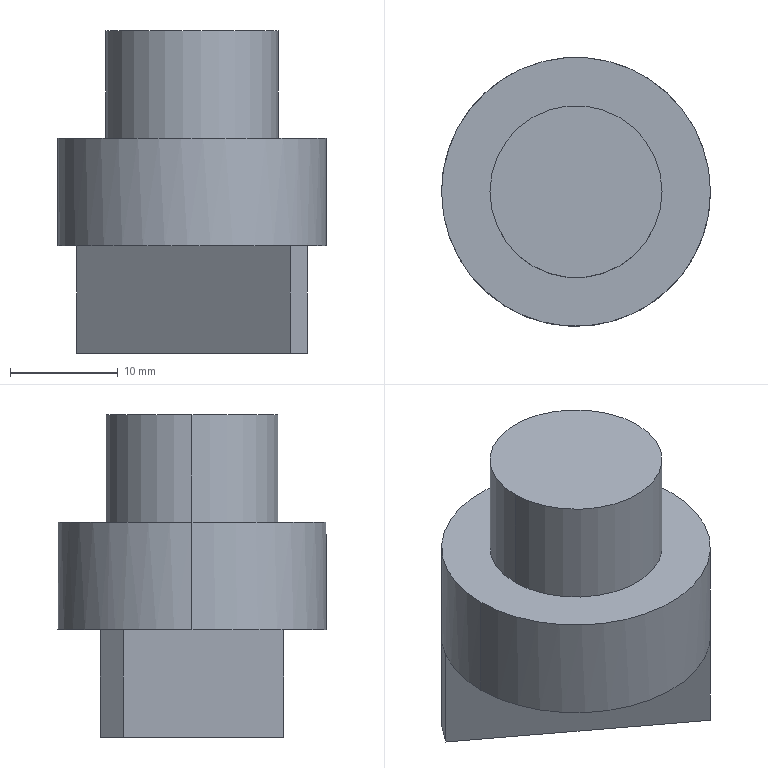Part | STEP file | Selector switch | 1 solid | 15 faces | box 25 x 25 x 30 mm | volume 7576 mm3 | plane 11 | cylinder 4 | commonest cylinder face diameters 16 x2 25 x2
STEP:
#1=CARTESIAN_POINT('',(0.,0.,0.));
#2=DIRECTION('',(0.,0.,1.));
#3=DIRECTION('',(1.,0.,0.));
#4=AXIS2_PLACEMENT_3D('',#1,#2,#3);
#5=CARTESIAN_POINT('',(-12.5,0.,10.));
#6=VERTEX_POINT('',#5);
#7=CARTESIAN_POINT('',(12.5,0.,10.));
#8=VERTEX_POINT('',#7);
#9=CARTESIAN_POINT('',(0.,0.,10.));
#10=DIRECTION('',(0.,0.,-1.));
#11=DIRECTION('',(-1.,0.,0.));
#12=AXIS2_PLACEMENT_3D('',#9,#10,#11);
#13=CIRCLE('',#12,12.5);
#14=CARTESIAN_POINT('',(0.,0.,10.));
#15=DIRECTION('',(0.,0.,-1.));
#16=DIRECTION('',(-1.,0.,0.));
#17=AXIS2_PLACEMENT_3D('',#14,#15,#16);
#18=CYLINDRICAL_SURFACE('',#17,12.5);
#19=CARTESIAN_POINT('',(0.,0.));
#20=DIRECTION('',(1.,0.));
#21=VECTOR('',#20,1.);
#22=LINE('',#19,#21);
#23=(GEOMETRIC_REPRESENTATION_CONTEXT(2)PARAMETRIC_REPRESENTATION_CONTEXT()REPRESENTATION_CONTEXT('',''));
#24=DEFINITIONAL_REPRESENTATION('',(#22),#23);
#25=PCURVE('',#18,#24);
#26=CARTESIAN_POINT('',(0.,0.,10.));
#27=DIRECTION('',(0.,0.,1.));
#28=DIRECTION('',(1.,0.,0.));
#29=AXIS2_PLACEMENT_3D('',#26,#27,#28);
#30=PLANE('',#29);
#31=CARTESIAN_POINT('',(-12.5,0.));
#32=CARTESIAN_POINT('',(-12.5,21.651));
#33=CARTESIAN_POINT('',(6.25,10.825));
#34=CARTESIAN_POINT('',(25.,0.));
#35=CARTESIAN_POINT('',(6.25,-10.825));
#36=CARTESIAN_POINT('',(-12.5,-21.651));
#37=CARTESIAN_POINT('',(-12.5,0.));
#38=(BOUNDED_CURVE()B_SPLINE_CURVE(2,(#31,#32,#33,#34,#35,#36,#37),.UNSPECIFIED.,.T.,.F.)B_SPLINE_CURVE_WITH_KNOTS((1,2,2,2,2,1),(-2.094,0.,2.094,4.189,6.283,8.378),.UNSPECIFIED.)CURVE()GEOMETRIC_REPRESENTATION_ITEM()RATIONAL_B_SPLINE_CURVE((1.,0.5,1.,0.5,1.,0.5,1.))REPRESENTATION_ITEM(''));
#39=(GEOMETRIC_REPRESENTATION_CONTEXT(2)PARAMETRIC_REPRESENTATION_CONTEXT()REPRESENTATION_CONTEXT('',''));
#40=DEFINITIONAL_REPRESENTATION('',(#38),#39);
#41=PCURVE('',#30,#40);
#42=SURFACE_CURVE('',#13,(#25,#41),.PCURVE_S1.);
#43=EDGE_CURVE('',#6,#8,#42,.T.);
#44=ORIENTED_EDGE('',*,*,#43,.T.);
#45=CARTESIAN_POINT('',(12.5,0.,0.));
#46=VERTEX_POINT('',#45);
#47=CARTESIAN_POINT('',(12.5,0.,10.));
#48=DIRECTION('',(0.,0.,-1.));
#49=VECTOR('',#48,1.);
#50=LINE('',#47,#49);
#51=CARTESIAN_POINT('',(3.142,0.));
#52=DIRECTION('',(0.,1.));
#53=VECTOR('',#52,1.);
#54=LINE('',#51,#53);
#55=(GEOMETRIC_REPRESENTATION_CONTEXT(2)PARAMETRIC_REPRESENTATION_CONTEXT()REPRESENTATION_CONTEXT('',''));
#56=DEFINITIONAL_REPRESENTATION('',(#54),#55);
#57=PCURVE('',#18,#56);
#58=CARTESIAN_POINT('',(0.,0.,10.));
#59=DIRECTION('',(0.,0.,-1.));
#60=DIRECTION('',(-1.,0.,0.));
#61=AXIS2_PLACEMENT_3D('',#58,#59,#60);
#62=CYLINDRICAL_SURFACE('',#61,12.5);
#63=CARTESIAN_POINT('',(3.142,0.));
#64=DIRECTION('',(0.,1.));
#65=VECTOR('',#64,1.);
#66=LINE('',#63,#65);
#67=(GEOMETRIC_REPRESENTATION_CONTEXT(2)PARAMETRIC_REPRESENTATION_CONTEXT()REPRESENTATION_CONTEXT('',''));
#68=DEFINITIONAL_REPRESENTATION('',(#66),#67);
#69=PCURVE('',#62,#68);
#70=SURFACE_CURVE('',#50,(#57,#69),.PCURVE_S1.);
#71=EDGE_CURVE('',#8,#46,#70,.T.);
#72=ORIENTED_EDGE('',*,*,#71,.T.);
#73=CARTESIAN_POINT('',(-9.149,8.518,0.));
#74=VERTEX_POINT('',#73);
#75=CARTESIAN_POINT('',(0.,0.,0.));
#76=DIRECTION('',(0.,0.,1.));
#77=DIRECTION('',(-1.,0.,0.));
#78=AXIS2_PLACEMENT_3D('',#75,#76,#77);
#79=CIRCLE('',#78,12.5);
#80=CARTESIAN_POINT('',(6.283,10.));
#81=DIRECTION('',(-1.,0.));
#82=VECTOR('',#81,1.);
#83=LINE('',#80,#82);
#84=(GEOMETRIC_REPRESENTATION_CONTEXT(2)PARAMETRIC_REPRESENTATION_CONTEXT()REPRESENTATION_CONTEXT('',''));
#85=DEFINITIONAL_REPRESENTATION('',(#83),#84);
#86=PCURVE('',#18,#85);
#87=CARTESIAN_POINT('',(0.,0.,0.));
#88=DIRECTION('',(0.,0.,1.));
#89=DIRECTION('',(1.,0.,0.));
#90=AXIS2_PLACEMENT_3D('',#87,#88,#89);
#91=PLANE('',#90);
#92=CARTESIAN_POINT('',(0.,0.));
#93=DIRECTION('',(-1.,0.));
#94=AXIS2_PLACEMENT_2D('',#92,#93);
#95=CIRCLE('',#94,12.5);
#96=(GEOMETRIC_REPRESENTATION_CONTEXT(2)PARAMETRIC_REPRESENTATION_CONTEXT()REPRESENTATION_CONTEXT('',''));
#97=DEFINITIONAL_REPRESENTATION('',(#95),#96);
#98=PCURVE('',#91,#97);
#99=SURFACE_CURVE('',#79,(#86,#98),.PCURVE_S1.);
#100=EDGE_CURVE('',#46,#74,#99,.T.);
#101=ORIENTED_EDGE('',*,*,#100,.T.);
#102=CARTESIAN_POINT('',(-10.733,6.406,0.));
#103=VERTEX_POINT('',#102);
#104=CARTESIAN_POINT('',(0.,0.,0.));
#105=DIRECTION('',(0.,0.,1.));
#106=DIRECTION('',(-1.,0.,0.));
#107=AXIS2_PLACEMENT_3D('',#104,#105,#106);
#108=CIRCLE('',#107,12.5);
#109=CARTESIAN_POINT('',(6.283,10.));
#110=DIRECTION('',(-1.,0.));
#111=VECTOR('',#110,1.);
#112=LINE('',#109,#111);
#113=(GEOMETRIC_REPRESENTATION_CONTEXT(2)PARAMETRIC_REPRESENTATION_CONTEXT()REPRESENTATION_CONTEXT('',''));
#114=DEFINITIONAL_REPRESENTATION('',(#112),#113);
#115=PCURVE('',#18,#114);
#116=CARTESIAN_POINT('',(0.,0.,0.));
#117=DIRECTION('',(0.,0.,1.));
#118=DIRECTION('',(1.,0.,0.));
#119=AXIS2_PLACEMENT_3D('',#116,#117,#118);
#120=PLANE('',#119);
#121=CARTESIAN_POINT('',(0.,0.));
#122=DIRECTION('',(-1.,0.));
#123=AXIS2_PLACEMENT_2D('',#121,#122);
#124=CIRCLE('',#123,12.5);
#125=(GEOMETRIC_REPRESENTATION_CONTEXT(2)PARAMETRIC_REPRESENTATION_CONTEXT()REPRESENTATION_CONTEXT('',''));
#126=DEFINITIONAL_REPRESENTATION('',(#124),#125);
#127=PCURVE('',#120,#126);
#128=SURFACE_CURVE('',#108,(#115,#127),.PCURVE_S1.);
#129=EDGE_CURVE('',#74,#103,#128,.T.);
#130=ORIENTED_EDGE('',*,*,#129,.T.);
#131=CARTESIAN_POINT('',(-12.5,0.,0.));
#132=VERTEX_POINT('',#131);
#133=CARTESIAN_POINT('',(0.,0.,0.));
#134=DIRECTION('',(0.,0.,1.));
#135=DIRECTION('',(-1.,0.,0.));
#136=AXIS2_PLACEMENT_3D('',#133,#134,#135);
#137=CIRCLE('',#136,12.5);
#138=CARTESIAN_POINT('',(6.283,10.));
#139=DIRECTION('',(-1.,0.));
#140=VECTOR('',#139,1.);
#141=LINE('',#138,#140);
#142=(GEOMETRIC_REPRESENTATION_CONTEXT(2)PARAMETRIC_REPRESENTATION_CONTEXT()REPRESENTATION_CONTEXT('',''));
#143=DEFINITIONAL_REPRESENTATION('',(#141),#142);
#144=PCURVE('',#18,#143);
#145=CARTESIAN_POINT('',(0.,0.,0.));
#146=DIRECTION('',(0.,0.,1.));
#147=DIRECTION('',(1.,0.,0.));
#148=AXIS2_PLACEMENT_3D('',#145,#146,#147);
#149=PLANE('',#148);
#150=CARTESIAN_POINT('',(0.,0.));
#151=DIRECTION('',(-1.,0.));
#152=AXIS2_PLACEMENT_2D('',#150,#151);
#153=CIRCLE('',#152,12.5);
#154=(GEOMETRIC_REPRESENTATION_CONTEXT(2)PARAMETRIC_REPRESENTATION_CONTEXT()REPRESENTATION_CONTEXT('',''));
#155=DEFINITIONAL_REPRESENTATION('',(#153),#154);
#156=PCURVE('',#149,#155);
#157=SURFACE_CURVE('',#137,(#144,#156),.PCURVE_S1.);
#158=EDGE_CURVE('',#103,#132,#157,.T.);
#159=ORIENTED_EDGE('',*,*,#158,.T.);
#160=CARTESIAN_POINT('',(-12.5,0.,10.));
#161=DIRECTION('',(0.,0.,-1.));
#162=VECTOR('',#161,1.);
#163=LINE('',#160,#162);
#164=CARTESIAN_POINT('',(0.,0.));
#165=DIRECTION('',(0.,1.));
#166=VECTOR('',#165,1.);
#167=LINE('',#164,#166);
#168=(GEOMETRIC_REPRESENTATION_CONTEXT(2)PARAMETRIC_REPRESENTATION_CONTEXT()REPRESENTATION_CONTEXT('',''));
#169=DEFINITIONAL_REPRESENTATION('',(#167),#168);
#170=PCURVE('',#18,#169);
#171=CARTESIAN_POINT('',(6.283,0.));
#172=DIRECTION('',(0.,1.));
#173=VECTOR('',#172,1.);
#174=LINE('',#171,#173);
#175=(GEOMETRIC_REPRESENTATION_CONTEXT(2)PARAMETRIC_REPRESENTATION_CONTEXT()REPRESENTATION_CONTEXT('',''));
#176=DEFINITIONAL_REPRESENTATION('',(#174),#175);
#177=PCURVE('',#62,#176);
#178=SURFACE_CURVE('',#163,(#170,#177),.PCURVE_S1.);
#179=EDGE_CURVE('',#6,#132,#178,.T.);
#180=ORIENTED_EDGE('',*,*,#179,.F.);
#181=EDGE_LOOP('',(#44,#72,#101,#130,#159,#180));
#182=FACE_BOUND('',#181,.T.);
#183=ADVANCED_FACE('',(#182),#18,.T.);
#184=CARTESIAN_POINT('',(-8.,0.,20.));
#185=VERTEX_POINT('',#184);
#186=CARTESIAN_POINT('',(8.,0.,20.));
#187=VERTEX_POINT('',#186);
#188=CARTESIAN_POINT('',(0.,0.,20.));
#189=DIRECTION('',(0.,0.,-1.));
#190=DIRECTION('',(-1.,0.,0.));
#191=AXIS2_PLACEMENT_3D('',#188,#189,#190);
#192=CIRCLE('',#191,8.);
#193=CARTESIAN_POINT('',(0.,0.,20.));
#194=DIRECTION('',(0.,0.,-1.));
#195=DIRECTION('',(-1.,0.,0.));
#196=AXIS2_PLACEMENT_3D('',#193,#194,#195);
#197=CYLINDRICAL_SURFACE('',#196,8.);
#198=CARTESIAN_POINT('',(0.,0.));
#199=DIRECTION('',(1.,0.));
#200=VECTOR('',#199,1.);
#201=LINE('',#198,#200);
#202=(GEOMETRIC_REPRESENTATION_CONTEXT(2)PARAMETRIC_REPRESENTATION_CONTEXT()REPRESENTATION_CONTEXT('',''));
#203=DEFINITIONAL_REPRESENTATION('',(#201),#202);
#204=PCURVE('',#197,#203);
#205=CARTESIAN_POINT('',(0.,0.,20.));
#206=DIRECTION('',(0.,0.,1.));
#207=DIRECTION('',(1.,0.,0.));
#208=AXIS2_PLACEMENT_3D('',#205,#206,#207);
#209=PLANE('',#208);
#210=CARTESIAN_POINT('',(-8.,0.));
#211=CARTESIAN_POINT('',(-8.,13.856));
#212=CARTESIAN_POINT('',(4.,6.928));
#213=CARTESIAN_POINT('',(16.,0.));
#214=CARTESIAN_POINT('',(4.,-6.928));
#215=CARTESIAN_POINT('',(-8.,-13.856));
#216=CARTESIAN_POINT('',(-8.,0.));
#217=(BOUNDED_CURVE()B_SPLINE_CURVE(2,(#210,#211,#212,#213,#214,#215,#216),.UNSPECIFIED.,.T.,.F.)B_SPLINE_CURVE_WITH_KNOTS((1,2,2,2,2,1),(-2.094,0.,2.094,4.189,6.283,8.378),.UNSPECIFIED.)CURVE()GEOMETRIC_REPRESENTATION_ITEM()RATIONAL_B_SPLINE_CURVE((1.,0.5,1.,0.5,1.,0.5,1.))REPRESENTATION_ITEM(''));
#218=(GEOMETRIC_REPRESENTATION_CONTEXT(2)PARAMETRIC_REPRESENTATION_CONTEXT()REPRESENTATION_CONTEXT('',''));
#219=DEFINITIONAL_REPRESENTATION('',(#217),#218);
#220=PCURVE('',#209,#219);
#221=SURFACE_CURVE('',#192,(#204,#220),.PCURVE_S1.);
#222=EDGE_CURVE('',#185,#187,#221,.T.);
#223=ORIENTED_EDGE('',*,*,#222,.T.);
#224=CARTESIAN_POINT('',(8.,0.,10.));
#225=VERTEX_POINT('',#224);
#226=CARTESIAN_POINT('',(8.,0.,20.));
#227=DIRECTION('',(0.,0.,-1.));
#228=VECTOR('',#227,1.);
#229=LINE('',#226,#228);
#230=CARTESIAN_POINT('',(3.142,0.));
#231=DIRECTION('',(0.,1.));
#232=VECTOR('',#231,1.);
#233=LINE('',#230,#232);
#234=(GEOMETRIC_REPRESENTATION_CONTEXT(2)PARAMETRIC_REPRESENTATION_CONTEXT()REPRESENTATION_CONTEXT('',''));
#235=DEFINITIONAL_REPRESENTATION('',(#233),#234);
#236=PCURVE('',#197,#235);
#237=CARTESIAN_POINT('',(0.,0.,20.));
#238=DIRECTION('',(0.,0.,-1.));
#239=DIRECTION('',(-1.,0.,0.));
#240=AXIS2_PLACEMENT_3D('',#237,#238,#239);
#241=CYLINDRICAL_SURFACE('',#240,8.);
#242=CARTESIAN_POINT('',(3.142,0.));
#243=DIRECTION('',(0.,1.));
#244=VECTOR('',#243,1.);
#245=LINE('',#242,#244);
#246=(GEOMETRIC_REPRESENTATION_CONTEXT(2)PARAMETRIC_REPRESENTATION_CONTEXT()REPRESENTATION_CONTEXT('',''));
#247=DEFINITIONAL_REPRESENTATION('',(#245),#246);
#248=PCURVE('',#241,#247);
#249=SURFACE_CURVE('',#229,(#236,#248),.PCURVE_S1.);
#250=EDGE_CURVE('',#187,#225,#249,.T.);
#251=ORIENTED_EDGE('',*,*,#250,.T.);
#252=CARTESIAN_POINT('',(-8.,0.,10.));
#253=VERTEX_POINT('',#252);
#254=CARTESIAN_POINT('',(0.,0.,10.));
#255=DIRECTION('',(0.,0.,-1.));
#256=DIRECTION('',(-1.,0.,0.));
#257=AXIS2_PLACEMENT_3D('',#254,#255,#256);
#258=CIRCLE('',#257,8.);
#259=CARTESIAN_POINT('',(0.,10.));
#260=DIRECTION('',(1.,0.));
#261=VECTOR('',#260,1.);
#262=LINE('',#259,#261);
#263=(GEOMETRIC_REPRESENTATION_CONTEXT(2)PARAMETRIC_REPRESENTATION_CONTEXT()REPRESENTATION_CONTEXT('',''));
#264=DEFINITIONAL_REPRESENTATION('',(#262),#263);
#265=PCURVE('',#197,#264);
#266=CARTESIAN_POINT('',(-8.,0.));
#267=CARTESIAN_POINT('',(-8.,13.856));
#268=CARTESIAN_POINT('',(4.,6.928));
#269=CARTESIAN_POINT('',(16.,0.));
#270=CARTESIAN_POINT('',(4.,-6.928));
#271=CARTESIAN_POINT('',(-8.,-13.856));
#272=CARTESIAN_POINT('',(-8.,0.));
#273=(BOUNDED_CURVE()B_SPLINE_CURVE(2,(#266,#267,#268,#269,#270,#271,#272),.UNSPECIFIED.,.T.,.F.)B_SPLINE_CURVE_WITH_KNOTS((1,2,2,2,2,1),(-2.094,0.,2.094,4.189,6.283,8.378),.UNSPECIFIED.)CURVE()GEOMETRIC_REPRESENTATION_ITEM()RATIONAL_B_SPLINE_CURVE((1.,0.5,1.,0.5,1.,0.5,1.))REPRESENTATION_ITEM(''));
#274=(GEOMETRIC_REPRESENTATION_CONTEXT(2)PARAMETRIC_REPRESENTATION_CONTEXT()REPRESENTATION_CONTEXT('',''));
#275=DEFINITIONAL_REPRESENTATION('',(#273),#274);
#276=PCURVE('',#30,#275);
#277=SURFACE_CURVE('',#258,(#265,#276),.PCURVE_S1.);
#278=EDGE_CURVE('',#253,#225,#277,.T.);
#279=ORIENTED_EDGE('',*,*,#278,.F.);
#280=CARTESIAN_POINT('',(-8.,0.,20.));
#281=DIRECTION('',(0.,0.,-1.));
#282=VECTOR('',#281,1.);
#283=LINE('',#280,#282);
#284=CARTESIAN_POINT('',(0.,0.));
#285=DIRECTION('',(0.,1.));
#286=VECTOR('',#285,1.);
#287=LINE('',#284,#286);
#288=(GEOMETRIC_REPRESENTATION_CONTEXT(2)PARAMETRIC_REPRESENTATION_CONTEXT()REPRESENTATION_CONTEXT('',''));
#289=DEFINITIONAL_REPRESENTATION('',(#287),#288);
#290=PCURVE('',#197,#289);
#291=CARTESIAN_POINT('',(6.283,0.));
#292=DIRECTION('',(0.,1.));
#293=VECTOR('',#292,1.);
#294=LINE('',#291,#293);
#295=(GEOMETRIC_REPRESENTATION_CONTEXT(2)PARAMETRIC_REPRESENTATION_CONTEXT()REPRESENTATION_CONTEXT('',''));
#296=DEFINITIONAL_REPRESENTATION('',(#294),#295);
#297=PCURVE('',#241,#296);
#298=SURFACE_CURVE('',#283,(#290,#297),.PCURVE_S1.);
#299=EDGE_CURVE('',#185,#253,#298,.T.);
#300=ORIENTED_EDGE('',*,*,#299,.F.);
#301=EDGE_LOOP('',(#223,#251,#279,#300));
#302=FACE_BOUND('',#301,.T.);
#303=ADVANCED_FACE('',(#302),#197,.T.);
#304=ORIENTED_EDGE('',*,*,#71,.F.);
#305=CARTESIAN_POINT('',(0.,0.,10.));
#306=DIRECTION('',(0.,0.,-1.));
#307=DIRECTION('',(-1.,0.,0.));
#308=AXIS2_PLACEMENT_3D('',#305,#306,#307);
#309=CIRCLE('',#308,12.5);
#310=CARTESIAN_POINT('',(0.,0.));
#311=DIRECTION('',(1.,0.));
#312=VECTOR('',#311,1.);
#313=LINE('',#310,#312);
#314=(GEOMETRIC_REPRESENTATION_CONTEXT(2)PARAMETRIC_REPRESENTATION_CONTEXT()REPRESENTATION_CONTEXT('',''));
#315=DEFINITIONAL_REPRESENTATION('',(#313),#314);
#316=PCURVE('',#62,#315);
#317=CARTESIAN_POINT('',(-12.5,0.));
#318=CARTESIAN_POINT('',(-12.5,21.651));
#319=CARTESIAN_POINT('',(6.25,10.825));
#320=CARTESIAN_POINT('',(25.,0.));
#321=CARTESIAN_POINT('',(6.25,-10.825));
#322=CARTESIAN_POINT('',(-12.5,-21.651));
#323=CARTESIAN_POINT('',(-12.5,0.));
#324=(BOUNDED_CURVE()B_SPLINE_CURVE(2,(#317,#318,#319,#320,#321,#322,#323),.UNSPECIFIED.,.T.,.F.)B_SPLINE_CURVE_WITH_KNOTS((1,2,2,2,2,1),(-2.094,0.,2.094,4.189,6.283,8.378),.UNSPECIFIED.)CURVE()GEOMETRIC_REPRESENTATION_ITEM()RATIONAL_B_SPLINE_CURVE((1.,0.5,1.,0.5,1.,0.5,1.))REPRESENTATION_ITEM(''));
#325=(GEOMETRIC_REPRESENTATION_CONTEXT(2)PARAMETRIC_REPRESENTATION_CONTEXT()REPRESENTATION_CONTEXT('',''));
#326=DEFINITIONAL_REPRESENTATION('',(#324),#325);
#327=PCURVE('',#30,#326);
#328=SURFACE_CURVE('',#309,(#316,#327),.PCURVE_S1.);
#329=EDGE_CURVE('',#8,#6,#328,.T.);
#330=ORIENTED_EDGE('',*,*,#329,.T.);
#331=ORIENTED_EDGE('',*,*,#179,.T.);
#332=CARTESIAN_POINT('',(9.149,-8.518,0.));
#333=VERTEX_POINT('',#332);
#334=CARTESIAN_POINT('',(0.,0.,0.));
#335=DIRECTION('',(0.,0.,1.));
#336=DIRECTION('',(-1.,0.,0.));
#337=AXIS2_PLACEMENT_3D('',#334,#335,#336);
#338=CIRCLE('',#337,12.5);
#339=CARTESIAN_POINT('',(6.283,10.));
#340=DIRECTION('',(-1.,0.));
#341=VECTOR('',#340,1.);
#342=LINE('',#339,#341);
#343=(GEOMETRIC_REPRESENTATION_CONTEXT(2)PARAMETRIC_REPRESENTATION_CONTEXT()REPRESENTATION_CONTEXT('',''));
#344=DEFINITIONAL_REPRESENTATION('',(#342),#343);
#345=PCURVE('',#62,#344);
#346=CARTESIAN_POINT('',(0.,0.));
#347=DIRECTION('',(-1.,0.));
#348=AXIS2_PLACEMENT_2D('',#346,#347);
#349=CIRCLE('',#348,12.5);
#350=(GEOMETRIC_REPRESENTATION_CONTEXT(2)PARAMETRIC_REPRESENTATION_CONTEXT()REPRESENTATION_CONTEXT('',''));
#351=DEFINITIONAL_REPRESENTATION('',(#349),#350);
#352=PCURVE('',#149,#351);
#353=SURFACE_CURVE('',#338,(#345,#352),.PCURVE_S1.);
#354=EDGE_CURVE('',#132,#333,#353,.T.);
#355=ORIENTED_EDGE('',*,*,#354,.T.);
#356=CARTESIAN_POINT('',(10.733,-6.406,0.));
#357=VERTEX_POINT('',#356);
#358=CARTESIAN_POINT('',(0.,0.,0.));
#359=DIRECTION('',(0.,0.,1.));
#360=DIRECTION('',(-1.,0.,0.));
#361=AXIS2_PLACEMENT_3D('',#358,#359,#360);
#362=CIRCLE('',#361,12.5);
#363=CARTESIAN_POINT('',(6.283,10.));
#364=DIRECTION('',(-1.,0.));
#365=VECTOR('',#364,1.);
#366=LINE('',#363,#365);
#367=(GEOMETRIC_REPRESENTATION_CONTEXT(2)PARAMETRIC_REPRESENTATION_CONTEXT()REPRESENTATION_CONTEXT('',''));
#368=DEFINITIONAL_REPRESENTATION('',(#366),#367);
#369=PCURVE('',#62,#368);
#370=CARTESIAN_POINT('',(0.,0.,0.));
#371=DIRECTION('',(0.,0.,1.));
#372=DIRECTION('',(1.,0.,0.));
#373=AXIS2_PLACEMENT_3D('',#370,#371,#372);
#374=PLANE('',#373);
#375=CARTESIAN_POINT('',(0.,0.));
#376=DIRECTION('',(-1.,0.));
#377=AXIS2_PLACEMENT_2D('',#375,#376);
#378=CIRCLE('',#377,12.5);
#379=(GEOMETRIC_REPRESENTATION_CONTEXT(2)PARAMETRIC_REPRESENTATION_CONTEXT()REPRESENTATION_CONTEXT('',''));
#380=DEFINITIONAL_REPRESENTATION('',(#378),#379);
#381=PCURVE('',#374,#380);
#382=SURFACE_CURVE('',#362,(#369,#381),.PCURVE_S1.);
#383=EDGE_CURVE('',#333,#357,#382,.T.);
#384=ORIENTED_EDGE('',*,*,#383,.T.);
#385=CARTESIAN_POINT('',(0.,0.,0.));
#386=DIRECTION('',(0.,0.,1.));
#387=DIRECTION('',(-1.,0.,0.));
#388=AXIS2_PLACEMENT_3D('',#385,#386,#387);
#389=CIRCLE('',#388,12.5);
#390=CARTESIAN_POINT('',(6.283,10.));
#391=DIRECTION('',(-1.,0.));
#392=VECTOR('',#391,1.);
#393=LINE('',#390,#392);
#394=(GEOMETRIC_REPRESENTATION_CONTEXT(2)PARAMETRIC_REPRESENTATION_CONTEXT()REPRESENTATION_CONTEXT('',''));
#395=DEFINITIONAL_REPRESENTATION('',(#393),#394);
#396=PCURVE('',#62,#395);
#397=CARTESIAN_POINT('',(0.,0.));
#398=DIRECTION('',(-1.,0.));
#399=AXIS2_PLACEMENT_2D('',#397,#398);
#400=CIRCLE('',#399,12.5);
#401=(GEOMETRIC_REPRESENTATION_CONTEXT(2)PARAMETRIC_REPRESENTATION_CONTEXT()REPRESENTATION_CONTEXT('',''));
#402=DEFINITIONAL_REPRESENTATION('',(#400),#401);
#403=PCURVE('',#91,#402);
#404=SURFACE_CURVE('',#389,(#396,#403),.PCURVE_S1.);
#405=EDGE_CURVE('',#357,#46,#404,.T.);
#406=ORIENTED_EDGE('',*,*,#405,.T.);
#407=EDGE_LOOP('',(#304,#330,#331,#355,#384,#406));
#408=FACE_BOUND('',#407,.T.);
#409=ADVANCED_FACE('',(#408),#62,.T.);
#410=CARTESIAN_POINT('',(-9.149,8.518,0.));
#411=DIRECTION('',(0.7998,-0.6003,0.));
#412=VECTOR('',#411,1.);
#413=LINE('',#410,#412);
#414=CARTESIAN_POINT('',(-9.149,8.518));
#415=DIRECTION('',(0.7998,-0.6003));
#416=VECTOR('',#415,1.);
#417=LINE('',#414,#416);
#418=(GEOMETRIC_REPRESENTATION_CONTEXT(2)PARAMETRIC_REPRESENTATION_CONTEXT()REPRESENTATION_CONTEXT('',''));
#419=DEFINITIONAL_REPRESENTATION('',(#417),#418);
#420=PCURVE('',#91,#419);
#421=CARTESIAN_POINT('',(-9.149,8.518,-10.));
#422=DIRECTION('',(-0.6003,-0.7998,0.));
#423=DIRECTION('',(0.7998,-0.6003,0.));
#424=AXIS2_PLACEMENT_3D('',#421,#422,#423);
#425=PLANE('',#424);
#426=CARTESIAN_POINT('',(0.,10.));
#427=DIRECTION('',(1.,0.));
#428=VECTOR('',#427,1.);
#429=LINE('',#426,#428);
#430=(GEOMETRIC_REPRESENTATION_CONTEXT(2)PARAMETRIC_REPRESENTATION_CONTEXT()REPRESENTATION_CONTEXT('',''));
#431=DEFINITIONAL_REPRESENTATION('',(#429),#430);
#432=PCURVE('',#425,#431);
#433=SURFACE_CURVE('',#413,(#420,#432),.PCURVE_S1.);
#434=EDGE_CURVE('',#74,#357,#433,.T.);
#435=ORIENTED_EDGE('',*,*,#434,.F.);
#436=ORIENTED_EDGE('',*,*,#100,.F.);
#437=ORIENTED_EDGE('',*,*,#405,.F.);
#438=EDGE_LOOP('',(#435,#436,#437));
#439=FACE_BOUND('',#438,.T.);
#440=ADVANCED_FACE('',(#439),#91,.F.);
#441=ORIENTED_EDGE('',*,*,#383,.F.);
#442=CARTESIAN_POINT('',(10.733,-6.406,0.));
#443=DIRECTION('',(-0.6003,-0.7998,0.));
#444=VECTOR('',#443,1.);
#445=LINE('',#442,#444);
#446=CARTESIAN_POINT('',(10.733,-6.406));
#447=DIRECTION('',(-0.6003,-0.7998));
#448=VECTOR('',#447,1.);
#449=LINE('',#446,#448);
#450=(GEOMETRIC_REPRESENTATION_CONTEXT(2)PARAMETRIC_REPRESENTATION_CONTEXT()REPRESENTATION_CONTEXT('',''));
#451=DEFINITIONAL_REPRESENTATION('',(#449),#450);
#452=PCURVE('',#374,#451);
#453=CARTESIAN_POINT('',(10.733,-6.406,-10.));
#454=DIRECTION('',(-0.7998,0.6003,0.));
#455=DIRECTION('',(-0.6003,-0.7998,0.));
#456=AXIS2_PLACEMENT_3D('',#453,#454,#455);
#457=PLANE('',#456);
#458=CARTESIAN_POINT('',(0.,10.));
#459=DIRECTION('',(1.,0.));
#460=VECTOR('',#459,1.);
#461=LINE('',#458,#460);
#462=(GEOMETRIC_REPRESENTATION_CONTEXT(2)PARAMETRIC_REPRESENTATION_CONTEXT()REPRESENTATION_CONTEXT('',''));
#463=DEFINITIONAL_REPRESENTATION('',(#461),#462);
#464=PCURVE('',#457,#463);
#465=SURFACE_CURVE('',#445,(#452,#464),.PCURVE_S1.);
#466=EDGE_CURVE('',#357,#333,#465,.T.);
#467=ORIENTED_EDGE('',*,*,#466,.F.);
#468=EDGE_LOOP('',(#441,#467));
#469=FACE_BOUND('',#468,.T.);
#470=ADVANCED_FACE('',(#469),#374,.F.);
#471=ORIENTED_EDGE('',*,*,#158,.F.);
#472=CARTESIAN_POINT('',(9.149,-8.518,0.));
#473=DIRECTION('',(-0.7998,0.6003,0.));
#474=VECTOR('',#473,1.);
#475=LINE('',#472,#474);
#476=CARTESIAN_POINT('',(9.149,-8.518));
#477=DIRECTION('',(-0.7998,0.6003));
#478=VECTOR('',#477,1.);
#479=LINE('',#476,#478);
#480=(GEOMETRIC_REPRESENTATION_CONTEXT(2)PARAMETRIC_REPRESENTATION_CONTEXT()REPRESENTATION_CONTEXT('',''));
#481=DEFINITIONAL_REPRESENTATION('',(#479),#480);
#482=PCURVE('',#149,#481);
#483=CARTESIAN_POINT('',(9.149,-8.518,-10.));
#484=DIRECTION('',(0.6003,0.7998,0.));
#485=DIRECTION('',(-0.7998,0.6003,0.));
#486=AXIS2_PLACEMENT_3D('',#483,#484,#485);
#487=PLANE('',#486);
#488=CARTESIAN_POINT('',(0.,10.));
#489=DIRECTION('',(1.,0.));
#490=VECTOR('',#489,1.);
#491=LINE('',#488,#490);
#492=(GEOMETRIC_REPRESENTATION_CONTEXT(2)PARAMETRIC_REPRESENTATION_CONTEXT()REPRESENTATION_CONTEXT('',''));
#493=DEFINITIONAL_REPRESENTATION('',(#491),#492);
#494=PCURVE('',#487,#493);
#495=SURFACE_CURVE('',#475,(#482,#494),.PCURVE_S1.);
#496=EDGE_CURVE('',#333,#103,#495,.T.);
#497=ORIENTED_EDGE('',*,*,#496,.F.);
#498=ORIENTED_EDGE('',*,*,#354,.F.);
#499=EDGE_LOOP('',(#471,#497,#498));
#500=FACE_BOUND('',#499,.T.);
#501=ADVANCED_FACE('',(#500),#149,.F.);
#502=ORIENTED_EDGE('',*,*,#278,.T.);
#503=CARTESIAN_POINT('',(0.,0.,10.));
#504=DIRECTION('',(0.,0.,-1.));
#505=DIRECTION('',(-1.,0.,0.));
#506=AXIS2_PLACEMENT_3D('',#503,#504,#505);
#507=CIRCLE('',#506,8.);
#508=CARTESIAN_POINT('',(-8.,0.));
#509=CARTESIAN_POINT('',(-8.,13.856));
#510=CARTESIAN_POINT('',(4.,6.928));
#511=CARTESIAN_POINT('',(16.,0.));
#512=CARTESIAN_POINT('',(4.,-6.928));
#513=CARTESIAN_POINT('',(-8.,-13.856));
#514=CARTESIAN_POINT('',(-8.,0.));
#515=(BOUNDED_CURVE()B_SPLINE_CURVE(2,(#508,#509,#510,#511,#512,#513,#514),.UNSPECIFIED.,.T.,.F.)B_SPLINE_CURVE_WITH_KNOTS((1,2,2,2,2,1),(-2.094,0.,2.094,4.189,6.283,8.378),.UNSPECIFIED.)CURVE()GEOMETRIC_REPRESENTATION_ITEM()RATIONAL_B_SPLINE_CURVE((1.,0.5,1.,0.5,1.,0.5,1.))REPRESENTATION_ITEM(''));
#516=(GEOMETRIC_REPRESENTATION_CONTEXT(2)PARAMETRIC_REPRESENTATION_CONTEXT()REPRESENTATION_CONTEXT('',''));
#517=DEFINITIONAL_REPRESENTATION('',(#515),#516);
#518=PCURVE('',#30,#517);
#519=CARTESIAN_POINT('',(0.,10.));
#520=DIRECTION('',(1.,0.));
#521=VECTOR('',#520,1.);
#522=LINE('',#519,#521);
#523=(GEOMETRIC_REPRESENTATION_CONTEXT(2)PARAMETRIC_REPRESENTATION_CONTEXT()REPRESENTATION_CONTEXT('',''));
#524=DEFINITIONAL_REPRESENTATION('',(#522),#523);
#525=PCURVE('',#241,#524);
#526=SURFACE_CURVE('',#507,(#518,#525),.PCURVE_S1.);
#527=EDGE_CURVE('',#225,#253,#526,.T.);
#528=ORIENTED_EDGE('',*,*,#527,.T.);
#529=EDGE_LOOP('',(#502,#528));
#530=FACE_BOUND('',#529,.T.);
#531=ORIENTED_EDGE('',*,*,#43,.F.);
#532=ORIENTED_EDGE('',*,*,#329,.F.);
#533=EDGE_LOOP('',(#531,#532));
#534=FACE_BOUND('',#533,.T.);
#535=ADVANCED_FACE('',(#530,#534),#30,.T.);
#536=CARTESIAN_POINT('',(10.733,-6.406,-10.));
#537=VERTEX_POINT('',#536);
#538=CARTESIAN_POINT('',(10.733,-6.406,-10.));
#539=DIRECTION('',(0.,0.,1.));
#540=VECTOR('',#539,1.);
#541=LINE('',#538,#540);
#542=CARTESIAN_POINT('',(24.86,0.));
#543=DIRECTION('',(0.,1.));
#544=VECTOR('',#543,1.);
#545=LINE('',#542,#544);
#546=(GEOMETRIC_REPRESENTATION_CONTEXT(2)PARAMETRIC_REPRESENTATION_CONTEXT()REPRESENTATION_CONTEXT('',''));
#547=DEFINITIONAL_REPRESENTATION('',(#545),#546);
#548=PCURVE('',#425,#547);
#549=CARTESIAN_POINT('',(0.,0.));
#550=DIRECTION('',(0.,1.));
#551=VECTOR('',#550,1.);
#552=LINE('',#549,#551);
#553=(GEOMETRIC_REPRESENTATION_CONTEXT(2)PARAMETRIC_REPRESENTATION_CONTEXT()REPRESENTATION_CONTEXT('',''));
#554=DEFINITIONAL_REPRESENTATION('',(#552),#553);
#555=PCURVE('',#457,#554);
#556=SURFACE_CURVE('',#541,(#548,#555),.PCURVE_S1.);
#557=EDGE_CURVE('',#537,#357,#556,.T.);
#558=ORIENTED_EDGE('',*,*,#557,.F.);
#559=CARTESIAN_POINT('',(-9.149,8.518,-10.));
#560=VERTEX_POINT('',#559);
#561=CARTESIAN_POINT('',(-9.149,8.518,-10.));
#562=DIRECTION('',(0.7998,-0.6003,0.));
#563=VECTOR('',#562,1.);
#564=LINE('',#561,#563);
#565=CARTESIAN_POINT('',(0.,0.));
#566=DIRECTION('',(1.,0.));
#567=VECTOR('',#566,1.);
#568=LINE('',#565,#567);
#569=(GEOMETRIC_REPRESENTATION_CONTEXT(2)PARAMETRIC_REPRESENTATION_CONTEXT()REPRESENTATION_CONTEXT('',''));
#570=DEFINITIONAL_REPRESENTATION('',(#568),#569);
#571=PCURVE('',#425,#570);
#572=CARTESIAN_POINT('',(-10.733,6.406,-10.));
#573=DIRECTION('',(0.,0.,-1.));
#574=DIRECTION('',(-1.,0.,0.));
#575=AXIS2_PLACEMENT_3D('',#572,#573,#574);
#576=PLANE('',#575);
#577=CARTESIAN_POINT('',(-1.585,2.111));
#578=DIRECTION('',(-0.7998,-0.6003));
#579=VECTOR('',#578,1.);
#580=LINE('',#577,#579);
#581=(GEOMETRIC_REPRESENTATION_CONTEXT(2)PARAMETRIC_REPRESENTATION_CONTEXT()REPRESENTATION_CONTEXT('',''));
#582=DEFINITIONAL_REPRESENTATION('',(#580),#581);
#583=PCURVE('',#576,#582);
#584=SURFACE_CURVE('',#564,(#571,#583),.PCURVE_S1.);
#585=EDGE_CURVE('',#560,#537,#584,.T.);
#586=ORIENTED_EDGE('',*,*,#585,.F.);
#587=CARTESIAN_POINT('',(-9.149,8.518,-10.));
#588=DIRECTION('',(0.,0.,-1.));
#589=VECTOR('',#588,1.);
#590=LINE('',#587,#589);
#591=CARTESIAN_POINT('',(0.,0.));
#592=DIRECTION('',(0.,-1.));
#593=VECTOR('',#592,1.);
#594=LINE('',#591,#593);
#595=(GEOMETRIC_REPRESENTATION_CONTEXT(2)PARAMETRIC_REPRESENTATION_CONTEXT()REPRESENTATION_CONTEXT('',''));
#596=DEFINITIONAL_REPRESENTATION('',(#594),#595);
#597=PCURVE('',#425,#596);
#598=CARTESIAN_POINT('',(-9.149,8.518,-10.));
#599=DIRECTION('',(0.7998,-0.6003,0.));
#600=DIRECTION('',(0.6003,0.7998,0.));
#601=AXIS2_PLACEMENT_3D('',#598,#599,#600);
#602=PLANE('',#601);
#603=CARTESIAN_POINT('',(0.,0.));
#604=DIRECTION('',(0.,-1.));
#605=VECTOR('',#604,1.);
#606=LINE('',#603,#605);
#607=(GEOMETRIC_REPRESENTATION_CONTEXT(2)PARAMETRIC_REPRESENTATION_CONTEXT()REPRESENTATION_CONTEXT('',''));
#608=DEFINITIONAL_REPRESENTATION('',(#606),#607);
#609=PCURVE('',#602,#608);
#610=SURFACE_CURVE('',#590,(#597,#609),.PCURVE_S1.);
#611=EDGE_CURVE('',#74,#560,#610,.T.);
#612=ORIENTED_EDGE('',*,*,#611,.F.);
#613=ORIENTED_EDGE('',*,*,#434,.T.);
#614=EDGE_LOOP('',(#558,#586,#612,#613));
#615=FACE_BOUND('',#614,.T.);
#616=ADVANCED_FACE('',(#615),#425,.F.);
#617=CARTESIAN_POINT('',(9.149,-8.518,-10.));
#618=VERTEX_POINT('',#617);
#619=CARTESIAN_POINT('',(9.149,-8.518,-10.));
#620=DIRECTION('',(0.,0.,1.));
#621=VECTOR('',#620,1.);
#622=LINE('',#619,#621);
#623=CARTESIAN_POINT('',(2.64,0.));
#624=DIRECTION('',(0.,1.));
#625=VECTOR('',#624,1.);
#626=LINE('',#623,#625);
#627=(GEOMETRIC_REPRESENTATION_CONTEXT(2)PARAMETRIC_REPRESENTATION_CONTEXT()REPRESENTATION_CONTEXT('',''));
#628=DEFINITIONAL_REPRESENTATION('',(#626),#627);
#629=PCURVE('',#457,#628);
#630=CARTESIAN_POINT('',(0.,0.));
#631=DIRECTION('',(0.,1.));
#632=VECTOR('',#631,1.);
#633=LINE('',#630,#632);
#634=(GEOMETRIC_REPRESENTATION_CONTEXT(2)PARAMETRIC_REPRESENTATION_CONTEXT()REPRESENTATION_CONTEXT('',''));
#635=DEFINITIONAL_REPRESENTATION('',(#633),#634);
#636=PCURVE('',#487,#635);
#637=SURFACE_CURVE('',#622,(#629,#636),.PCURVE_S1.);
#638=EDGE_CURVE('',#618,#333,#637,.T.);
#639=ORIENTED_EDGE('',*,*,#638,.F.);
#640=CARTESIAN_POINT('',(10.733,-6.406,-10.));
#641=DIRECTION('',(-0.6003,-0.7998,0.));
#642=VECTOR('',#641,1.);
#643=LINE('',#640,#642);
#644=CARTESIAN_POINT('',(0.,0.));
#645=DIRECTION('',(1.,0.));
#646=VECTOR('',#645,1.);
#647=LINE('',#644,#646);
#648=(GEOMETRIC_REPRESENTATION_CONTEXT(2)PARAMETRIC_REPRESENTATION_CONTEXT()REPRESENTATION_CONTEXT('',''));
#649=DEFINITIONAL_REPRESENTATION('',(#647),#648);
#650=PCURVE('',#457,#649);
#651=CARTESIAN_POINT('',(-21.467,-12.813));
#652=DIRECTION('',(0.6003,-0.7998));
#653=VECTOR('',#652,1.);
#654=LINE('',#651,#653);
#655=(GEOMETRIC_REPRESENTATION_CONTEXT(2)PARAMETRIC_REPRESENTATION_CONTEXT()REPRESENTATION_CONTEXT('',''));
#656=DEFINITIONAL_REPRESENTATION('',(#654),#655);
#657=PCURVE('',#576,#656);
#658=SURFACE_CURVE('',#643,(#650,#657),.PCURVE_S1.);
#659=EDGE_CURVE('',#537,#618,#658,.T.);
#660=ORIENTED_EDGE('',*,*,#659,.F.);
#661=ORIENTED_EDGE('',*,*,#557,.T.);
#662=ORIENTED_EDGE('',*,*,#466,.T.);
#663=EDGE_LOOP('',(#639,#660,#661,#662));
#664=FACE_BOUND('',#663,.T.);
#665=ADVANCED_FACE('',(#664),#457,.F.);
#666=CARTESIAN_POINT('',(-10.733,6.406,-10.));
#667=VERTEX_POINT('',#666);
#668=CARTESIAN_POINT('',(-10.733,6.406,-10.));
#669=DIRECTION('',(0.,0.,1.));
#670=VECTOR('',#669,1.);
#671=LINE('',#668,#670);
#672=CARTESIAN_POINT('',(24.86,0.));
#673=DIRECTION('',(0.,1.));
#674=VECTOR('',#673,1.);
#675=LINE('',#672,#674);
#676=(GEOMETRIC_REPRESENTATION_CONTEXT(2)PARAMETRIC_REPRESENTATION_CONTEXT()REPRESENTATION_CONTEXT('',''));
#677=DEFINITIONAL_REPRESENTATION('',(#675),#676);
#678=PCURVE('',#487,#677);
#679=CARTESIAN_POINT('',(-2.64,0.));
#680=DIRECTION('',(0.,1.));
#681=VECTOR('',#680,1.);
#682=LINE('',#679,#681);
#683=(GEOMETRIC_REPRESENTATION_CONTEXT(2)PARAMETRIC_REPRESENTATION_CONTEXT()REPRESENTATION_CONTEXT('',''));
#684=DEFINITIONAL_REPRESENTATION('',(#682),#683);
#685=PCURVE('',#602,#684);
#686=SURFACE_CURVE('',#671,(#678,#685),.PCURVE_S1.);
#687=EDGE_CURVE('',#667,#103,#686,.T.);
#688=ORIENTED_EDGE('',*,*,#687,.F.);
#689=CARTESIAN_POINT('',(9.149,-8.518,-10.));
#690=DIRECTION('',(-0.7998,0.6003,0.));
#691=VECTOR('',#690,1.);
#692=LINE('',#689,#691);
#693=CARTESIAN_POINT('',(0.,0.));
#694=DIRECTION('',(1.,0.));
#695=VECTOR('',#694,1.);
#696=LINE('',#693,#695);
#697=(GEOMETRIC_REPRESENTATION_CONTEXT(2)PARAMETRIC_REPRESENTATION_CONTEXT()REPRESENTATION_CONTEXT('',''));
#698=DEFINITIONAL_REPRESENTATION('',(#696),#697);
#699=PCURVE('',#487,#698);
#700=CARTESIAN_POINT('',(-19.882,-14.924));
#701=DIRECTION('',(0.7998,0.6003));
#702=VECTOR('',#701,1.);
#703=LINE('',#700,#702);
#704=(GEOMETRIC_REPRESENTATION_CONTEXT(2)PARAMETRIC_REPRESENTATION_CONTEXT()REPRESENTATION_CONTEXT('',''));
#705=DEFINITIONAL_REPRESENTATION('',(#703),#704);
#706=PCURVE('',#576,#705);
#707=SURFACE_CURVE('',#692,(#699,#706),.PCURVE_S1.);
#708=EDGE_CURVE('',#618,#667,#707,.T.);
#709=ORIENTED_EDGE('',*,*,#708,.F.);
#710=ORIENTED_EDGE('',*,*,#638,.T.);
#711=ORIENTED_EDGE('',*,*,#496,.T.);
#712=EDGE_LOOP('',(#688,#709,#710,#711));
#713=FACE_BOUND('',#712,.T.);
#714=ADVANCED_FACE('',(#713),#487,.F.);
#715=ORIENTED_EDGE('',*,*,#129,.F.);
#716=CARTESIAN_POINT('',(-10.733,6.406,0.));
#717=DIRECTION('',(0.6003,0.7998,0.));
#718=VECTOR('',#717,1.);
#719=LINE('',#716,#718);
#720=CARTESIAN_POINT('',(-10.733,6.406));
#721=DIRECTION('',(0.6003,0.7998));
#722=VECTOR('',#721,1.);
#723=LINE('',#720,#722);
#724=(GEOMETRIC_REPRESENTATION_CONTEXT(2)PARAMETRIC_REPRESENTATION_CONTEXT()REPRESENTATION_CONTEXT('',''));
#725=DEFINITIONAL_REPRESENTATION('',(#723),#724);
#726=PCURVE('',#120,#725);
#727=CARTESIAN_POINT('',(-2.64,10.));
#728=DIRECTION('',(1.,0.));
#729=VECTOR('',#728,1.);
#730=LINE('',#727,#729);
#731=(GEOMETRIC_REPRESENTATION_CONTEXT(2)PARAMETRIC_REPRESENTATION_CONTEXT()REPRESENTATION_CONTEXT('',''));
#732=DEFINITIONAL_REPRESENTATION('',(#730),#731);
#733=PCURVE('',#602,#732);
#734=SURFACE_CURVE('',#719,(#726,#733),.PCURVE_S1.);
#735=EDGE_CURVE('',#103,#74,#734,.T.);
#736=ORIENTED_EDGE('',*,*,#735,.F.);
#737=EDGE_LOOP('',(#715,#736));
#738=FACE_BOUND('',#737,.T.);
#739=ADVANCED_FACE('',(#738),#120,.F.);
#740=ORIENTED_EDGE('',*,*,#250,.F.);
#741=CARTESIAN_POINT('',(0.,0.,20.));
#742=DIRECTION('',(0.,0.,-1.));
#743=DIRECTION('',(-1.,0.,0.));
#744=AXIS2_PLACEMENT_3D('',#741,#742,#743);
#745=CIRCLE('',#744,8.);
#746=CARTESIAN_POINT('',(0.,0.));
#747=DIRECTION('',(1.,0.));
#748=VECTOR('',#747,1.);
#749=LINE('',#746,#748);
#750=(GEOMETRIC_REPRESENTATION_CONTEXT(2)PARAMETRIC_REPRESENTATION_CONTEXT()REPRESENTATION_CONTEXT('',''));
#751=DEFINITIONAL_REPRESENTATION('',(#749),#750);
#752=PCURVE('',#241,#751);
#753=CARTESIAN_POINT('',(-8.,0.));
#754=CARTESIAN_POINT('',(-8.,13.856));
#755=CARTESIAN_POINT('',(4.,6.928));
#756=CARTESIAN_POINT('',(16.,0.));
#757=CARTESIAN_POINT('',(4.,-6.928));
#758=CARTESIAN_POINT('',(-8.,-13.856));
#759=CARTESIAN_POINT('',(-8.,0.));
#760=(BOUNDED_CURVE()B_SPLINE_CURVE(2,(#753,#754,#755,#756,#757,#758,#759),.UNSPECIFIED.,.T.,.F.)B_SPLINE_CURVE_WITH_KNOTS((1,2,2,2,2,1),(-2.094,0.,2.094,4.189,6.283,8.378),.UNSPECIFIED.)CURVE()GEOMETRIC_REPRESENTATION_ITEM()RATIONAL_B_SPLINE_CURVE((1.,0.5,1.,0.5,1.,0.5,1.))REPRESENTATION_ITEM(''));
#761=(GEOMETRIC_REPRESENTATION_CONTEXT(2)PARAMETRIC_REPRESENTATION_CONTEXT()REPRESENTATION_CONTEXT('',''));
#762=DEFINITIONAL_REPRESENTATION('',(#760),#761);
#763=PCURVE('',#209,#762);
#764=SURFACE_CURVE('',#745,(#752,#763),.PCURVE_S1.);
#765=EDGE_CURVE('',#187,#185,#764,.T.);
#766=ORIENTED_EDGE('',*,*,#765,.T.);
#767=ORIENTED_EDGE('',*,*,#299,.T.);
#768=ORIENTED_EDGE('',*,*,#527,.F.);
#769=EDGE_LOOP('',(#740,#766,#767,#768));
#770=FACE_BOUND('',#769,.T.);
#771=ADVANCED_FACE('',(#770),#241,.T.);
#772=ORIENTED_EDGE('',*,*,#659,.T.);
#773=ORIENTED_EDGE('',*,*,#708,.T.);
#774=CARTESIAN_POINT('',(-10.733,6.406,-10.));
#775=DIRECTION('',(0.6003,0.7998,0.));
#776=VECTOR('',#775,1.);
#777=LINE('',#774,#776);
#778=CARTESIAN_POINT('',(0.,0.));
#779=DIRECTION('',(-0.6003,0.7998));
#780=VECTOR('',#779,1.);
#781=LINE('',#778,#780);
#782=(GEOMETRIC_REPRESENTATION_CONTEXT(2)PARAMETRIC_REPRESENTATION_CONTEXT()REPRESENTATION_CONTEXT('',''));
#783=DEFINITIONAL_REPRESENTATION('',(#781),#782);
#784=PCURVE('',#576,#783);
#785=CARTESIAN_POINT('',(-2.64,0.));
#786=DIRECTION('',(1.,0.));
#787=VECTOR('',#786,1.);
#788=LINE('',#785,#787);
#789=(GEOMETRIC_REPRESENTATION_CONTEXT(2)PARAMETRIC_REPRESENTATION_CONTEXT()REPRESENTATION_CONTEXT('',''));
#790=DEFINITIONAL_REPRESENTATION('',(#788),#789);
#791=PCURVE('',#602,#790);
#792=SURFACE_CURVE('',#777,(#784,#791),.PCURVE_S1.);
#793=EDGE_CURVE('',#667,#560,#792,.T.);
#794=ORIENTED_EDGE('',*,*,#793,.T.);
#795=ORIENTED_EDGE('',*,*,#585,.T.);
#796=EDGE_LOOP('',(#772,#773,#794,#795));
#797=FACE_BOUND('',#796,.T.);
#798=ADVANCED_FACE('',(#797),#576,.T.);
#799=ORIENTED_EDGE('',*,*,#611,.T.);
#800=ORIENTED_EDGE('',*,*,#793,.F.);
#801=ORIENTED_EDGE('',*,*,#687,.T.);
#802=ORIENTED_EDGE('',*,*,#735,.T.);
#803=EDGE_LOOP('',(#799,#800,#801,#802));
#804=FACE_BOUND('',#803,.T.);
#805=ADVANCED_FACE('',(#804),#602,.F.);
#806=ORIENTED_EDGE('',*,*,#222,.F.);
#807=ORIENTED_EDGE('',*,*,#765,.F.);
#808=EDGE_LOOP('',(#806,#807));
#809=FACE_BOUND('',#808,.T.);
#810=ADVANCED_FACE('',(#809),#209,.T.);
#811=CLOSED_SHELL('',(#183,#303,#409,#440,#470,#501,#535,#616,#665,#714,#739,#771,#798,#805,#810));
#812=MANIFOLD_SOLID_BREP('',#811);
#813=(LENGTH_UNIT()NAMED_UNIT(*)SI_UNIT(.MILLI.,.METRE.));
#814=UNCERTAINTY_MEASURE_WITH_UNIT(LENGTH_MEASURE(0.0000001),#813,'','');
#815=(NAMED_UNIT(*)PLANE_ANGLE_UNIT()SI_UNIT($,.RADIAN.));
#816=(NAMED_UNIT(*)SI_UNIT($,.STERADIAN.)SOLID_ANGLE_UNIT());
#817=(GEOMETRIC_REPRESENTATION_CONTEXT(3)GLOBAL_UNCERTAINTY_ASSIGNED_CONTEXT((#814))GLOBAL_UNIT_ASSIGNED_CONTEXT((#813,#815,#816))REPRESENTATION_CONTEXT('',''));
#818=ADVANCED_BREP_SHAPE_REPRESENTATION('',(#4,#812),#817);